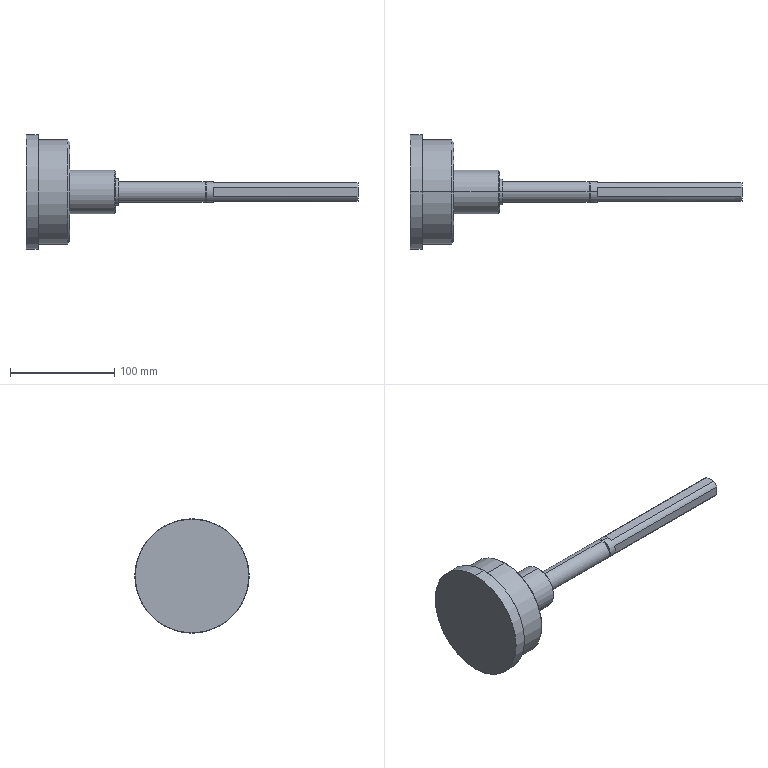Part | STEP file | film pull wheel_SUS304 | 1 solid | 42 faces | box 319 x 110 x 110 mm | volume 479492 mm3 | cylinder 16 | plane 16 | cone 10 | commonest cylinder face diameters 20 x4 6.8 x2 18.85 x2 25 x2 42 x2 100 x2